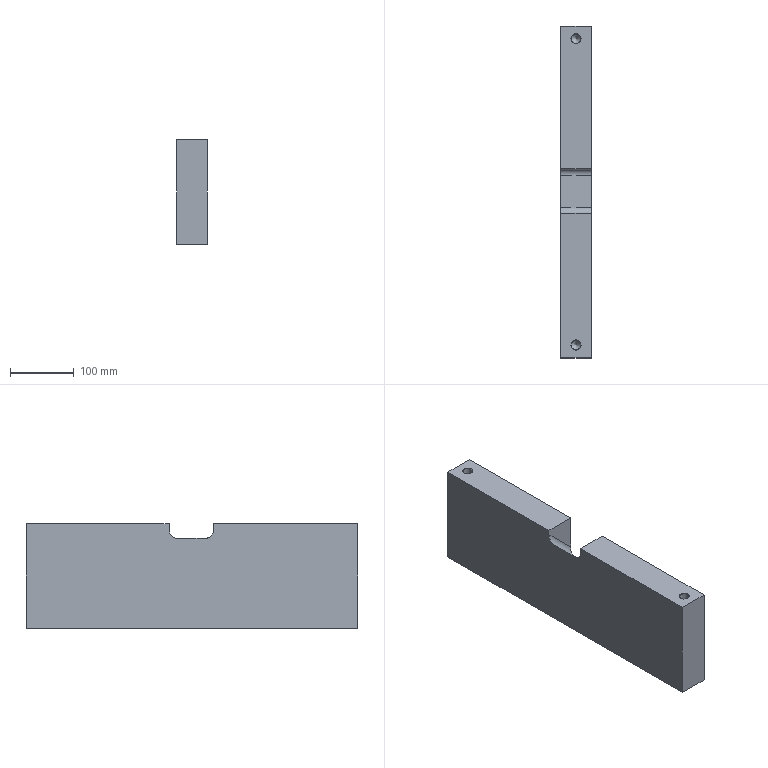Part | NX | features B2-6 2 | 1 solid | 24 faces | box 48 x 520 x 163 mm | volume 3875521 mm3 | plane 10 | cone 8 | cylinder 6 | commonest cylinder face diameters 14.506 x4 20 x2
STEP:
#1=CARTESIAN_POINT('',(3967.094,-1119.122,733.716));
#2=VERTEX_POINT('',#1);
#3=CARTESIAN_POINT('',(3967.094,-893.122,733.716));
#4=VERTEX_POINT('',#3);
#5=CARTESIAN_POINT('',(3967.094,-859.122,733.716));
#6=DIRECTION('',(0.,1.,0.));
#7=VECTOR('',#6,1000.);
#8=LINE('',#5,#7);
#9=EDGE_CURVE('',#2,#4,#8,.T.);
#10=ORIENTED_EDGE('',*,*,#9,.T.);
#11=CARTESIAN_POINT('',(3967.094,-893.122,725.858));
#12=VERTEX_POINT('',#11);
#13=CARTESIAN_POINT('',(3967.094,-893.122,793.716));
#14=DIRECTION('',(0.,0.,-1.));
#15=VECTOR('',#14,1000.);
#16=LINE('',#13,#15);
#17=EDGE_CURVE('',#4,#12,#16,.T.);
#18=ORIENTED_EDGE('',*,*,#17,.T.);
#19=CARTESIAN_POINT('',(3967.094,-883.122,711.716));
#20=VERTEX_POINT('',#19);
#21=CARTESIAN_POINT('',(3967.094,-883.122,725.858));
#22=DIRECTION('',(1.,0.,0.));
#23=DIRECTION('',(0.,0.,1.));
#24=AXIS2_PLACEMENT_3D('',#21,#22,#23);
#25=ELLIPSE('',#24,14.142,10.);
#26=EDGE_CURVE('',#12,#20,#25,.T.);
#27=ORIENTED_EDGE('',*,*,#26,.T.);
#28=CARTESIAN_POINT('',(3967.094,-833.122,711.716));
#29=VERTEX_POINT('',#28);
#30=CARTESIAN_POINT('',(3967.094,-859.122,711.716));
#31=DIRECTION('',(0.,1.,0.));
#32=VECTOR('',#31,1000.);
#33=LINE('',#30,#32);
#34=EDGE_CURVE('',#29,#20,#33,.F.);
#35=ORIENTED_EDGE('',*,*,#34,.F.);
#36=CARTESIAN_POINT('',(3967.094,-823.122,725.858));
#37=VERTEX_POINT('',#36);
#38=CARTESIAN_POINT('',(3967.094,-833.122,725.858));
#39=DIRECTION('',(1.,0.,0.));
#40=DIRECTION('',(0.,0.,1.));
#41=AXIS2_PLACEMENT_3D('',#38,#39,#40);
#42=ELLIPSE('',#41,14.142,10.);
#43=EDGE_CURVE('',#29,#37,#42,.T.);
#44=ORIENTED_EDGE('',*,*,#43,.T.);
#45=CARTESIAN_POINT('',(3967.094,-823.122,733.716));
#46=VERTEX_POINT('',#45);
#47=CARTESIAN_POINT('',(3967.094,-823.122,793.716));
#48=DIRECTION('',(0.,0.,-1.));
#49=VECTOR('',#48,1000.);
#50=LINE('',#47,#49);
#51=EDGE_CURVE('',#37,#46,#50,.F.);
#52=ORIENTED_EDGE('',*,*,#51,.T.);
#53=CARTESIAN_POINT('',(3967.094,-599.122,733.716));
#54=VERTEX_POINT('',#53);
#55=CARTESIAN_POINT('',(3967.094,-859.122,733.716));
#56=DIRECTION('',(0.,1.,0.));
#57=VECTOR('',#56,1000.);
#58=LINE('',#55,#57);
#59=EDGE_CURVE('',#46,#54,#58,.T.);
#60=ORIENTED_EDGE('',*,*,#59,.T.);
#61=CARTESIAN_POINT('',(3967.094,-599.122,570.716));
#62=VERTEX_POINT('',#61);
#63=CARTESIAN_POINT('',(3967.094,-599.122,600.716));
#64=DIRECTION('',(0.,0.,1.));
#65=VECTOR('',#64,1000.);
#66=LINE('',#63,#65);
#67=EDGE_CURVE('',#62,#54,#66,.T.);
#68=ORIENTED_EDGE('',*,*,#67,.F.);
#69=CARTESIAN_POINT('',(3967.094,-1119.122,570.716));
#70=VERTEX_POINT('',#69);
#71=CARTESIAN_POINT('',(3967.094,0.,570.716));
#72=DIRECTION('',(0.,-1.,0.));
#73=VECTOR('',#72,1000.);
#74=LINE('',#71,#73);
#75=EDGE_CURVE('',#62,#70,#74,.T.);
#76=ORIENTED_EDGE('',*,*,#75,.T.);
#77=CARTESIAN_POINT('',(3967.094,-1119.122,600.716));
#78=DIRECTION('',(0.,0.,-1.));
#79=VECTOR('',#78,1000.);
#80=LINE('',#77,#79);
#81=EDGE_CURVE('',#2,#70,#80,.T.);
#82=ORIENTED_EDGE('',*,*,#81,.F.);
#83=EDGE_LOOP('',(#10,#18,#27,#35,#44,#52,#60,#68,#76,#82));
#84=FACE_BOUND('',#83,.T.);
#85=CARTESIAN_POINT('',(3967.094,-859.122,667.216));
#86=DIRECTION('',(1.,0.,0.));
#87=DIRECTION('',(0.,0.,-1.));
#88=AXIS2_PLACEMENT_3D('',#85,#86,#87);
#89=PLANE('',#88);
#90=ADVANCED_FACE('',(#84),#89,.F.);
#91=CARTESIAN_POINT('',(3999.094,-1099.122,733.716));
#92=VERTEX_POINT('',#91);
#93=CARTESIAN_POINT('',(3991.094,-1099.122,733.716));
#94=DIRECTION('',(0.,0.,1.));
#95=DIRECTION('',(1.,0.,0.));
#96=AXIS2_PLACEMENT_3D('',#93,#94,#95);
#97=CIRCLE('',#96,8.);
#98=EDGE_CURVE('',#92,#92,#97,.T.);
#99=ORIENTED_EDGE('',*,*,#98,.F.);
#100=EDGE_LOOP('',(#99));
#101=FACE_BOUND('',#100,.T.);
#102=CARTESIAN_POINT('',(4015.094,-893.122,733.716));
#103=VERTEX_POINT('',#102);
#104=CARTESIAN_POINT('',(-365.,-893.122,733.716));
#105=DIRECTION('',(1.,0.,0.));
#106=VECTOR('',#105,1000.);
#107=LINE('',#104,#106);
#108=EDGE_CURVE('',#103,#4,#107,.F.);
#109=ORIENTED_EDGE('',*,*,#108,.T.);
#110=ORIENTED_EDGE('',*,*,#9,.F.);
#111=CARTESIAN_POINT('',(4015.094,-1119.122,733.716));
#112=VERTEX_POINT('',#111);
#113=CARTESIAN_POINT('',(4015.094,-1119.122,733.716));
#114=DIRECTION('',(-1.,0.,0.));
#115=VECTOR('',#114,1000.);
#116=LINE('',#113,#115);
#117=EDGE_CURVE('',#112,#2,#116,.T.);
#118=ORIENTED_EDGE('',*,*,#117,.F.);
#119=CARTESIAN_POINT('',(4015.094,-599.122,733.716));
#120=DIRECTION('',(0.,-1.,0.));
#121=VECTOR('',#120,1000.);
#122=LINE('',#119,#121);
#123=EDGE_CURVE('',#103,#112,#122,.T.);
#124=ORIENTED_EDGE('',*,*,#123,.F.);
#125=EDGE_LOOP('',(#109,#110,#118,#124));
#126=FACE_BOUND('',#125,.T.);
#127=CARTESIAN_POINT('',(-365.,0.,733.716));
#128=DIRECTION('',(0.,0.,-1.));
#129=DIRECTION('',(-1.,0.,0.));
#130=AXIS2_PLACEMENT_3D('',#127,#128,#129);
#131=PLANE('',#130);
#132=ADVANCED_FACE('',(#101,#126),#131,.F.);
#133=CARTESIAN_POINT('',(4015.094,-823.122,677.858));
#134=VERTEX_POINT('',#133);
#135=CARTESIAN_POINT('',(4015.094,-823.122,733.716));
#136=VERTEX_POINT('',#135);
#137=CARTESIAN_POINT('',(4015.094,-823.122,600.716));
#138=DIRECTION('',(0.,0.,-1.));
#139=VECTOR('',#138,1000.);
#140=LINE('',#137,#139);
#141=EDGE_CURVE('',#134,#136,#140,.F.);
#142=ORIENTED_EDGE('',*,*,#141,.F.);
#143=CARTESIAN_POINT('',(4015.094,-833.122,663.716));
#144=VERTEX_POINT('',#143);
#145=CARTESIAN_POINT('',(4015.094,-833.122,677.858));
#146=DIRECTION('',(-1.,0.,0.));
#147=DIRECTION('',(0.,0.,1.));
#148=AXIS2_PLACEMENT_3D('',#145,#146,#147);
#149=ELLIPSE('',#148,14.142,10.);
#150=EDGE_CURVE('',#134,#144,#149,.T.);
#151=ORIENTED_EDGE('',*,*,#150,.T.);
#152=CARTESIAN_POINT('',(4015.094,-883.122,663.716));
#153=VERTEX_POINT('',#152);
#154=CARTESIAN_POINT('',(4015.094,-599.122,663.716));
#155=DIRECTION('',(0.,1.,0.));
#156=VECTOR('',#155,1000.);
#157=LINE('',#154,#156);
#158=EDGE_CURVE('',#144,#153,#157,.F.);
#159=ORIENTED_EDGE('',*,*,#158,.T.);
#160=CARTESIAN_POINT('',(4015.094,-893.122,677.858));
#161=VERTEX_POINT('',#160);
#162=CARTESIAN_POINT('',(4015.094,-883.122,677.858));
#163=DIRECTION('',(-1.,0.,0.));
#164=DIRECTION('',(0.,0.,1.));
#165=AXIS2_PLACEMENT_3D('',#162,#163,#164);
#166=ELLIPSE('',#165,14.142,10.);
#167=EDGE_CURVE('',#153,#161,#166,.T.);
#168=ORIENTED_EDGE('',*,*,#167,.T.);
#169=CARTESIAN_POINT('',(4015.094,-893.122,600.716));
#170=DIRECTION('',(0.,0.,-1.));
#171=VECTOR('',#170,1000.);
#172=LINE('',#169,#171);
#173=EDGE_CURVE('',#103,#161,#172,.T.);
#174=ORIENTED_EDGE('',*,*,#173,.F.);
#175=ORIENTED_EDGE('',*,*,#123,.T.);
#176=CARTESIAN_POINT('',(4015.094,-1119.122,570.716));
#177=VERTEX_POINT('',#176);
#178=CARTESIAN_POINT('',(4015.094,-1119.122,600.716));
#179=DIRECTION('',(0.,0.,1.));
#180=VECTOR('',#179,1000.);
#181=LINE('',#178,#180);
#182=EDGE_CURVE('',#177,#112,#181,.T.);
#183=ORIENTED_EDGE('',*,*,#182,.F.);
#184=CARTESIAN_POINT('',(4015.094,-599.122,570.716));
#185=VERTEX_POINT('',#184);
#186=CARTESIAN_POINT('',(4015.094,-599.122,570.716));
#187=DIRECTION('',(0.,-1.,0.));
#188=VECTOR('',#187,1000.);
#189=LINE('',#186,#188);
#190=EDGE_CURVE('',#185,#177,#189,.T.);
#191=ORIENTED_EDGE('',*,*,#190,.F.);
#192=CARTESIAN_POINT('',(4015.094,-599.122,733.716));
#193=VERTEX_POINT('',#192);
#194=CARTESIAN_POINT('',(4015.094,-599.122,600.716));
#195=DIRECTION('',(0.,0.,1.));
#196=VECTOR('',#195,1000.);
#197=LINE('',#194,#196);
#198=EDGE_CURVE('',#185,#193,#197,.T.);
#199=ORIENTED_EDGE('',*,*,#198,.T.);
#200=CARTESIAN_POINT('',(4015.094,-599.122,733.716));
#201=DIRECTION('',(0.,-1.,0.));
#202=VECTOR('',#201,1000.);
#203=LINE('',#200,#202);
#204=EDGE_CURVE('',#193,#136,#203,.T.);
#205=ORIENTED_EDGE('',*,*,#204,.T.);
#206=EDGE_LOOP('',(#142,#151,#159,#168,#174,#175,#183,#191,#199,#205));
#207=FACE_BOUND('',#206,.T.);
#208=CARTESIAN_POINT('',(4015.094,-599.122,600.716));
#209=DIRECTION('',(-1.,0.,0.));
#210=DIRECTION('',(0.,0.,1.));
#211=AXIS2_PLACEMENT_3D('',#208,#209,#210);
#212=PLANE('',#211);
#213=ADVANCED_FACE('',(#207),#212,.F.);
#214=CARTESIAN_POINT('',(3999.094,-619.122,733.716));
#215=VERTEX_POINT('',#214);
#216=CARTESIAN_POINT('',(3991.094,-619.122,733.716));
#217=DIRECTION('',(0.,0.,1.));
#218=DIRECTION('',(1.,0.,0.));
#219=AXIS2_PLACEMENT_3D('',#216,#217,#218);
#220=CIRCLE('',#219,8.);
#221=EDGE_CURVE('',#215,#215,#220,.T.);
#222=ORIENTED_EDGE('',*,*,#221,.F.);
#223=EDGE_LOOP('',(#222));
#224=FACE_BOUND('',#223,.T.);
#225=ORIENTED_EDGE('',*,*,#59,.F.);
#226=CARTESIAN_POINT('',(-365.,-823.122,733.716));
#227=DIRECTION('',(1.,0.,0.));
#228=VECTOR('',#227,1000.);
#229=LINE('',#226,#228);
#230=EDGE_CURVE('',#136,#46,#229,.F.);
#231=ORIENTED_EDGE('',*,*,#230,.F.);
#232=ORIENTED_EDGE('',*,*,#204,.F.);
#233=CARTESIAN_POINT('',(1890.094,-599.122,733.716));
#234=DIRECTION('',(1.,0.,0.));
#235=VECTOR('',#234,1000.);
#236=LINE('',#233,#235);
#237=EDGE_CURVE('',#54,#193,#236,.T.);
#238=ORIENTED_EDGE('',*,*,#237,.F.);
#239=EDGE_LOOP('',(#225,#231,#232,#238));
#240=FACE_BOUND('',#239,.T.);
#241=CARTESIAN_POINT('',(-365.,0.,733.716));
#242=DIRECTION('',(0.,0.,-1.));
#243=DIRECTION('',(-1.,0.,0.));
#244=AXIS2_PLACEMENT_3D('',#241,#242,#243);
#245=PLANE('',#244);
#246=ADVANCED_FACE('',(#224,#240),#245,.F.);
#247=CARTESIAN_POINT('',(3983.094,-1039.122,570.716));
#248=VERTEX_POINT('',#247);
#249=CARTESIAN_POINT('',(3991.094,-1039.122,570.716));
#250=DIRECTION('',(0.,0.,-1.));
#251=DIRECTION('',(-1.,0.,0.));
#252=AXIS2_PLACEMENT_3D('',#249,#250,#251);
#253=CIRCLE('',#252,8.);
#254=EDGE_CURVE('',#248,#248,#253,.T.);
#255=ORIENTED_EDGE('',*,*,#254,.F.);
#256=EDGE_LOOP('',(#255));
#257=FACE_BOUND('',#256,.T.);
#258=CARTESIAN_POINT('',(3983.094,-679.122,570.716));
#259=VERTEX_POINT('',#258);
#260=CARTESIAN_POINT('',(3991.094,-679.122,570.716));
#261=DIRECTION('',(0.,0.,-1.));
#262=DIRECTION('',(-1.,0.,0.));
#263=AXIS2_PLACEMENT_3D('',#260,#261,#262);
#264=CIRCLE('',#263,8.);
#265=EDGE_CURVE('',#259,#259,#264,.T.);
#266=ORIENTED_EDGE('',*,*,#265,.F.);
#267=EDGE_LOOP('',(#266));
#268=FACE_BOUND('',#267,.T.);
#269=CARTESIAN_POINT('',(4015.094,-1119.122,570.716));
#270=DIRECTION('',(-1.,0.,0.));
#271=VECTOR('',#270,1000.);
#272=LINE('',#269,#271);
#273=EDGE_CURVE('',#177,#70,#272,.T.);
#274=ORIENTED_EDGE('',*,*,#273,.T.);
#275=ORIENTED_EDGE('',*,*,#75,.F.);
#276=CARTESIAN_POINT('',(1890.094,-599.122,570.716));
#277=DIRECTION('',(1.,0.,0.));
#278=VECTOR('',#277,1000.);
#279=LINE('',#276,#278);
#280=EDGE_CURVE('',#62,#185,#279,.T.);
#281=ORIENTED_EDGE('',*,*,#280,.T.);
#282=ORIENTED_EDGE('',*,*,#190,.T.);
#283=EDGE_LOOP('',(#274,#275,#281,#282));
#284=FACE_BOUND('',#283,.T.);
#285=CARTESIAN_POINT('',(-365.,0.,570.716));
#286=DIRECTION('',(0.,0.,-1.));
#287=DIRECTION('',(-1.,0.,0.));
#288=AXIS2_PLACEMENT_3D('',#285,#286,#287);
#289=PLANE('',#288);
#290=ADVANCED_FACE('',(#257,#268,#284),#289,.T.);
#291=ORIENTED_EDGE('',*,*,#117,.T.);
#292=ORIENTED_EDGE('',*,*,#81,.T.);
#293=ORIENTED_EDGE('',*,*,#273,.F.);
#294=ORIENTED_EDGE('',*,*,#182,.T.);
#295=EDGE_LOOP('',(#291,#292,#293,#294));
#296=FACE_BOUND('',#295,.T.);
#297=CARTESIAN_POINT('',(4015.094,-1119.122,600.716));
#298=DIRECTION('',(0.,1.,0.));
#299=DIRECTION('',(-1.,0.,0.));
#300=AXIS2_PLACEMENT_3D('',#297,#298,#299);
#301=PLANE('',#300);
#302=ADVANCED_FACE('',(#296),#301,.F.);
#303=ORIENTED_EDGE('',*,*,#173,.T.);
#304=CARTESIAN_POINT('',(3972.165,-893.122,720.787));
#305=DIRECTION('',(0.7071,0.,-0.7071));
#306=VECTOR('',#305,1000.);
#307=LINE('',#304,#306);
#308=EDGE_CURVE('',#161,#12,#307,.F.);
#309=ORIENTED_EDGE('',*,*,#308,.T.);
#310=ORIENTED_EDGE('',*,*,#17,.F.);
#311=ORIENTED_EDGE('',*,*,#108,.F.);
#312=EDGE_LOOP('',(#303,#309,#310,#311));
#313=FACE_BOUND('',#312,.T.);
#314=CARTESIAN_POINT('',(4000.699,-893.122,793.716));
#315=DIRECTION('',(0.,1.,0.));
#316=DIRECTION('',(0.,0.,1.));
#317=AXIS2_PLACEMENT_3D('',#314,#315,#316);
#318=PLANE('',#317);
#319=ADVANCED_FACE('',(#313),#318,.T.);
#320=ORIENTED_EDGE('',*,*,#237,.T.);
#321=ORIENTED_EDGE('',*,*,#198,.F.);
#322=ORIENTED_EDGE('',*,*,#280,.F.);
#323=ORIENTED_EDGE('',*,*,#67,.T.);
#324=EDGE_LOOP('',(#320,#321,#322,#323));
#325=FACE_BOUND('',#324,.T.);
#326=CARTESIAN_POINT('',(1890.094,-599.122,600.716));
#327=DIRECTION('',(0.,-1.,0.));
#328=DIRECTION('',(0.,0.,-1.));
#329=AXIS2_PLACEMENT_3D('',#326,#327,#328);
#330=PLANE('',#329);
#331=ADVANCED_FACE('',(#325),#330,.F.);
#332=ORIENTED_EDGE('',*,*,#230,.T.);
#333=ORIENTED_EDGE('',*,*,#51,.F.);
#334=CARTESIAN_POINT('',(3942.468,-823.122,750.485));
#335=DIRECTION('',(-0.7071,0.,0.7071));
#336=VECTOR('',#335,1000.);
#337=LINE('',#334,#336);
#338=EDGE_CURVE('',#37,#134,#337,.F.);
#339=ORIENTED_EDGE('',*,*,#338,.T.);
#340=ORIENTED_EDGE('',*,*,#141,.T.);
#341=EDGE_LOOP('',(#332,#333,#339,#340));
#342=FACE_BOUND('',#341,.T.);
#343=CARTESIAN_POINT('',(4000.699,-823.122,793.716));
#344=DIRECTION('',(0.,1.,0.));
#345=DIRECTION('',(0.,0.,1.));
#346=AXIS2_PLACEMENT_3D('',#343,#344,#345);
#347=PLANE('',#346);
#348=ADVANCED_FACE('',(#342),#347,.F.);
#349=CARTESIAN_POINT('',(4000.094,-833.122,678.716));
#350=DIRECTION('',(0.7071,0.,-0.7071));
#351=VECTOR('',#350,1000.);
#352=LINE('',#349,#351);
#353=EDGE_CURVE('',#144,#29,#352,.F.);
#354=ORIENTED_EDGE('',*,*,#353,.T.);
#355=ORIENTED_EDGE('',*,*,#34,.T.);
#356=CARTESIAN_POINT('',(4000.094,-883.122,678.716));
#357=DIRECTION('',(-0.7071,0.,0.7071));
#358=VECTOR('',#357,1000.);
#359=LINE('',#356,#358);
#360=EDGE_CURVE('',#20,#153,#359,.F.);
#361=ORIENTED_EDGE('',*,*,#360,.T.);
#362=ORIENTED_EDGE('',*,*,#158,.F.);
#363=EDGE_LOOP('',(#354,#355,#361,#362));
#364=FACE_BOUND('',#363,.T.);
#365=CARTESIAN_POINT('',(4000.094,-599.122,678.716));
#366=DIRECTION('',(-0.7071,0.,-0.7071));
#367=DIRECTION('',(0.,-1.,0.));
#368=AXIS2_PLACEMENT_3D('',#365,#366,#367);
#369=PLANE('',#368);
#370=ADVANCED_FACE('',(#364),#369,.F.);
#371=ORIENTED_EDGE('',*,*,#26,.F.);
#372=ORIENTED_EDGE('',*,*,#308,.F.);
#373=ORIENTED_EDGE('',*,*,#167,.F.);
#374=ORIENTED_EDGE('',*,*,#360,.F.);
#375=EDGE_LOOP('',(#371,#372,#373,#374));
#376=FACE_BOUND('',#375,.T.);
#377=CARTESIAN_POINT('',(3942.468,-883.122,750.485));
#378=DIRECTION('',(-0.7071,0.,0.7071));
#379=DIRECTION('',(0.7071,0.,0.7071));
#380=AXIS2_PLACEMENT_3D('',#377,#378,#379);
#381=CYLINDRICAL_SURFACE('',#380,10.);
#382=ADVANCED_FACE('',(#376),#381,.F.);
#383=ORIENTED_EDGE('',*,*,#43,.F.);
#384=ORIENTED_EDGE('',*,*,#353,.F.);
#385=ORIENTED_EDGE('',*,*,#150,.F.);
#386=ORIENTED_EDGE('',*,*,#338,.F.);
#387=EDGE_LOOP('',(#383,#384,#385,#386));
#388=FACE_BOUND('',#387,.T.);
#389=CARTESIAN_POINT('',(3942.468,-833.122,750.485));
#390=DIRECTION('',(-0.7071,0.,0.7071));
#391=DIRECTION('',(0.7071,0.,0.7071));
#392=AXIS2_PLACEMENT_3D('',#389,#390,#391);
#393=CYLINDRICAL_SURFACE('',#392,10.);
#394=ADVANCED_FACE('',(#388),#393,.F.);
#395=CARTESIAN_POINT('',(3998.347,-1099.122,732.969));
#396=VERTEX_POINT('',#395);
#397=CARTESIAN_POINT('',(3991.094,-1099.122,732.969));
#398=DIRECTION('',(0.,0.,1.));
#399=DIRECTION('',(1.,0.,0.));
#400=AXIS2_PLACEMENT_3D('',#397,#398,#399);
#401=CIRCLE('',#400,7.253);
#402=EDGE_CURVE('',#396,#396,#401,.F.);
#403=ORIENTED_EDGE('',*,*,#402,.F.);
#404=EDGE_LOOP('',(#403));
#405=FACE_BOUND('',#404,.T.);
#406=CARTESIAN_POINT('',(3998.347,-1099.122,688.719));
#407=VERTEX_POINT('',#406);
#408=CARTESIAN_POINT('',(3991.094,-1099.122,688.719));
#409=DIRECTION('',(0.,0.,1.));
#410=DIRECTION('',(1.,0.,0.));
#411=AXIS2_PLACEMENT_3D('',#408,#409,#410);
#412=CIRCLE('',#411,7.253);
#413=EDGE_CURVE('',#407,#407,#412,.F.);
#414=ORIENTED_EDGE('',*,*,#413,.T.);
#415=EDGE_LOOP('',(#414));
#416=FACE_BOUND('',#415,.T.);
#417=CARTESIAN_POINT('',(3991.094,-1099.122,681.466));
#418=DIRECTION('',(0.,0.,1.));
#419=DIRECTION('',(1.,0.,0.));
#420=AXIS2_PLACEMENT_3D('',#417,#418,#419);
#421=CYLINDRICAL_SURFACE('',#420,7.253);
#422=ADVANCED_FACE('',(#405,#416),#421,.F.);
#423=CARTESIAN_POINT('',(3991.094,-1099.122,681.466));
#424=VERTEX_POINT('',#423);
#425=VERTEX_LOOP('',#424);
#426=FACE_BOUND('',#425,.T.);
#427=ORIENTED_EDGE('',*,*,#413,.F.);
#428=EDGE_LOOP('',(#427));
#429=FACE_BOUND('',#428,.T.);
#430=CARTESIAN_POINT('',(3991.094,-1099.122,688.716));
#431=DIRECTION('',(0.,0.,1.));
#432=DIRECTION('',(1.,0.,0.));
#433=AXIS2_PLACEMENT_3D('',#430,#431,#432);
#434=CONICAL_SURFACE('',#433,7.25,0.7854);
#435=ADVANCED_FACE('',(#426,#429),#434,.F.);
#436=ORIENTED_EDGE('',*,*,#402,.T.);
#437=EDGE_LOOP('',(#436));
#438=FACE_BOUND('',#437,.T.);
#439=ORIENTED_EDGE('',*,*,#98,.T.);
#440=EDGE_LOOP('',(#439));
#441=FACE_BOUND('',#440,.T.);
#442=CARTESIAN_POINT('',(3991.094,-1099.122,733.716));
#443=DIRECTION('',(0.,0.,1.));
#444=DIRECTION('',(1.,0.,0.));
#445=AXIS2_PLACEMENT_3D('',#442,#443,#444);
#446=CONICAL_SURFACE('',#445,8.,0.7854);
#447=ADVANCED_FACE('',(#438,#441),#446,.F.);
#448=CARTESIAN_POINT('',(3998.347,-619.122,732.969));
#449=VERTEX_POINT('',#448);
#450=CARTESIAN_POINT('',(3991.094,-619.122,732.969));
#451=DIRECTION('',(0.,0.,1.));
#452=DIRECTION('',(1.,0.,0.));
#453=AXIS2_PLACEMENT_3D('',#450,#451,#452);
#454=CIRCLE('',#453,7.253);
#455=EDGE_CURVE('',#449,#449,#454,.F.);
#456=ORIENTED_EDGE('',*,*,#455,.F.);
#457=EDGE_LOOP('',(#456));
#458=FACE_BOUND('',#457,.T.);
#459=CARTESIAN_POINT('',(3998.347,-619.122,688.719));
#460=VERTEX_POINT('',#459);
#461=CARTESIAN_POINT('',(3991.094,-619.122,688.719));
#462=DIRECTION('',(0.,0.,1.));
#463=DIRECTION('',(1.,0.,0.));
#464=AXIS2_PLACEMENT_3D('',#461,#462,#463);
#465=CIRCLE('',#464,7.253);
#466=EDGE_CURVE('',#460,#460,#465,.F.);
#467=ORIENTED_EDGE('',*,*,#466,.T.);
#468=EDGE_LOOP('',(#467));
#469=FACE_BOUND('',#468,.T.);
#470=CARTESIAN_POINT('',(3991.094,-619.122,681.466));
#471=DIRECTION('',(0.,0.,1.));
#472=DIRECTION('',(1.,0.,0.));
#473=AXIS2_PLACEMENT_3D('',#470,#471,#472);
#474=CYLINDRICAL_SURFACE('',#473,7.253);
#475=ADVANCED_FACE('',(#458,#469),#474,.F.);
#476=CARTESIAN_POINT('',(3991.094,-619.122,681.466));
#477=VERTEX_POINT('',#476);
#478=VERTEX_LOOP('',#477);
#479=FACE_BOUND('',#478,.T.);
#480=ORIENTED_EDGE('',*,*,#466,.F.);
#481=EDGE_LOOP('',(#480));
#482=FACE_BOUND('',#481,.T.);
#483=CARTESIAN_POINT('',(3991.094,-619.122,688.716));
#484=DIRECTION('',(0.,0.,1.));
#485=DIRECTION('',(1.,0.,0.));
#486=AXIS2_PLACEMENT_3D('',#483,#484,#485);
#487=CONICAL_SURFACE('',#486,7.25,0.7854);
#488=ADVANCED_FACE('',(#479,#482),#487,.F.);
#489=ORIENTED_EDGE('',*,*,#455,.T.);
#490=EDGE_LOOP('',(#489));
#491=FACE_BOUND('',#490,.T.);
#492=ORIENTED_EDGE('',*,*,#221,.T.);
#493=EDGE_LOOP('',(#492));
#494=FACE_BOUND('',#493,.T.);
#495=CARTESIAN_POINT('',(3991.094,-619.122,733.716));
#496=DIRECTION('',(0.,0.,1.));
#497=DIRECTION('',(1.,0.,0.));
#498=AXIS2_PLACEMENT_3D('',#495,#496,#497);
#499=CONICAL_SURFACE('',#498,8.,0.7854);
#500=ADVANCED_FACE('',(#491,#494),#499,.F.);
#501=CARTESIAN_POINT('',(3983.841,-679.122,571.463));
#502=VERTEX_POINT('',#501);
#503=CARTESIAN_POINT('',(3991.094,-679.122,571.463));
#504=DIRECTION('',(0.,0.,-1.));
#505=DIRECTION('',(-1.,0.,0.));
#506=AXIS2_PLACEMENT_3D('',#503,#504,#505);
#507=CIRCLE('',#506,7.253);
#508=EDGE_CURVE('',#502,#502,#507,.F.);
#509=ORIENTED_EDGE('',*,*,#508,.F.);
#510=EDGE_LOOP('',(#509));
#511=FACE_BOUND('',#510,.T.);
#512=CARTESIAN_POINT('',(3983.841,-679.122,645.713));
#513=VERTEX_POINT('',#512);
#514=CARTESIAN_POINT('',(3991.094,-679.122,645.713));
#515=DIRECTION('',(0.,0.,-1.));
#516=DIRECTION('',(-1.,0.,0.));
#517=AXIS2_PLACEMENT_3D('',#514,#515,#516);
#518=CIRCLE('',#517,7.253);
#519=EDGE_CURVE('',#513,#513,#518,.F.);
#520=ORIENTED_EDGE('',*,*,#519,.T.);
#521=EDGE_LOOP('',(#520));
#522=FACE_BOUND('',#521,.T.);
#523=CARTESIAN_POINT('',(3991.094,-679.122,652.966));
#524=DIRECTION('',(0.,0.,-1.));
#525=DIRECTION('',(-1.,0.,0.));
#526=AXIS2_PLACEMENT_3D('',#523,#524,#525);
#527=CYLINDRICAL_SURFACE('',#526,7.253);
#528=ADVANCED_FACE('',(#511,#522),#527,.F.);
#529=CARTESIAN_POINT('',(3991.094,-679.122,652.966));
#530=VERTEX_POINT('',#529);
#531=VERTEX_LOOP('',#530);
#532=FACE_BOUND('',#531,.T.);
#533=ORIENTED_EDGE('',*,*,#519,.F.);
#534=EDGE_LOOP('',(#533));
#535=FACE_BOUND('',#534,.T.);
#536=CARTESIAN_POINT('',(3991.094,-679.122,645.716));
#537=DIRECTION('',(0.,0.,-1.));
#538=DIRECTION('',(-1.,0.,0.));
#539=AXIS2_PLACEMENT_3D('',#536,#537,#538);
#540=CONICAL_SURFACE('',#539,7.25,0.7854);
#541=ADVANCED_FACE('',(#532,#535),#540,.F.);
#542=ORIENTED_EDGE('',*,*,#508,.T.);
#543=EDGE_LOOP('',(#542));
#544=FACE_BOUND('',#543,.T.);
#545=ORIENTED_EDGE('',*,*,#265,.T.);
#546=EDGE_LOOP('',(#545));
#547=FACE_BOUND('',#546,.T.);
#548=CARTESIAN_POINT('',(3991.094,-679.122,570.716));
#549=DIRECTION('',(0.,0.,-1.));
#550=DIRECTION('',(-1.,0.,0.));
#551=AXIS2_PLACEMENT_3D('',#548,#549,#550);
#552=CONICAL_SURFACE('',#551,8.,0.7854);
#553=ADVANCED_FACE('',(#544,#547),#552,.F.);
#554=CARTESIAN_POINT('',(3983.841,-1039.122,571.463));
#555=VERTEX_POINT('',#554);
#556=CARTESIAN_POINT('',(3991.094,-1039.122,571.463));
#557=DIRECTION('',(0.,0.,-1.));
#558=DIRECTION('',(-1.,0.,0.));
#559=AXIS2_PLACEMENT_3D('',#556,#557,#558);
#560=CIRCLE('',#559,7.253);
#561=EDGE_CURVE('',#555,#555,#560,.F.);
#562=ORIENTED_EDGE('',*,*,#561,.F.);
#563=EDGE_LOOP('',(#562));
#564=FACE_BOUND('',#563,.T.);
#565=CARTESIAN_POINT('',(3983.841,-1039.122,645.713));
#566=VERTEX_POINT('',#565);
#567=CARTESIAN_POINT('',(3991.094,-1039.122,645.713));
#568=DIRECTION('',(0.,0.,-1.));
#569=DIRECTION('',(-1.,0.,0.));
#570=AXIS2_PLACEMENT_3D('',#567,#568,#569);
#571=CIRCLE('',#570,7.253);
#572=EDGE_CURVE('',#566,#566,#571,.F.);
#573=ORIENTED_EDGE('',*,*,#572,.T.);
#574=EDGE_LOOP('',(#573));
#575=FACE_BOUND('',#574,.T.);
#576=CARTESIAN_POINT('',(3991.094,-1039.122,652.966));
#577=DIRECTION('',(0.,0.,-1.));
#578=DIRECTION('',(-1.,0.,0.));
#579=AXIS2_PLACEMENT_3D('',#576,#577,#578);
#580=CYLINDRICAL_SURFACE('',#579,7.253);
#581=ADVANCED_FACE('',(#564,#575),#580,.F.);
#582=CARTESIAN_POINT('',(3991.094,-1039.122,652.966));
#583=VERTEX_POINT('',#582);
#584=VERTEX_LOOP('',#583);
#585=FACE_BOUND('',#584,.T.);
#586=ORIENTED_EDGE('',*,*,#572,.F.);
#587=EDGE_LOOP('',(#586));
#588=FACE_BOUND('',#587,.T.);
#589=CARTESIAN_POINT('',(3991.094,-1039.122,645.716));
#590=DIRECTION('',(0.,0.,-1.));
#591=DIRECTION('',(-1.,0.,0.));
#592=AXIS2_PLACEMENT_3D('',#589,#590,#591);
#593=CONICAL_SURFACE('',#592,7.25,0.7854);
#594=ADVANCED_FACE('',(#585,#588),#593,.F.);
#595=ORIENTED_EDGE('',*,*,#561,.T.);
#596=EDGE_LOOP('',(#595));
#597=FACE_BOUND('',#596,.T.);
#598=ORIENTED_EDGE('',*,*,#254,.T.);
#599=EDGE_LOOP('',(#598));
#600=FACE_BOUND('',#599,.T.);
#601=CARTESIAN_POINT('',(3991.094,-1039.122,570.716));
#602=DIRECTION('',(0.,0.,-1.));
#603=DIRECTION('',(-1.,0.,0.));
#604=AXIS2_PLACEMENT_3D('',#601,#602,#603);
#605=CONICAL_SURFACE('',#604,8.,0.7854);
#606=ADVANCED_FACE('',(#597,#600),#605,.F.);
#607=CLOSED_SHELL('',(#90,#132,#213,#246,#290,#302,#319,#331,#348,#370,#382,#394,#422,#435,#447,#475,#488,#500,#528,#541,#553,#581,#594,#606));
#608=MANIFOLD_SOLID_BREP('',#607);
#609=(LENGTH_UNIT()NAMED_UNIT(*)SI_UNIT(.MILLI.,.METRE.));
#610=UNCERTAINTY_MEASURE_WITH_UNIT(LENGTH_MEASURE(0.00001),#609,'','');
#611=(NAMED_UNIT(*)PLANE_ANGLE_UNIT()SI_UNIT($,.RADIAN.));
#612=(NAMED_UNIT(*)SI_UNIT($,.STERADIAN.)SOLID_ANGLE_UNIT());
#613=(GEOMETRIC_REPRESENTATION_CONTEXT(3)GLOBAL_UNCERTAINTY_ASSIGNED_CONTEXT((#610))GLOBAL_UNIT_ASSIGNED_CONTEXT((#609,#611,#612))REPRESENTATION_CONTEXT('',''));
#614=ADVANCED_BREP_SHAPE_REPRESENTATION('',(#608),#613);